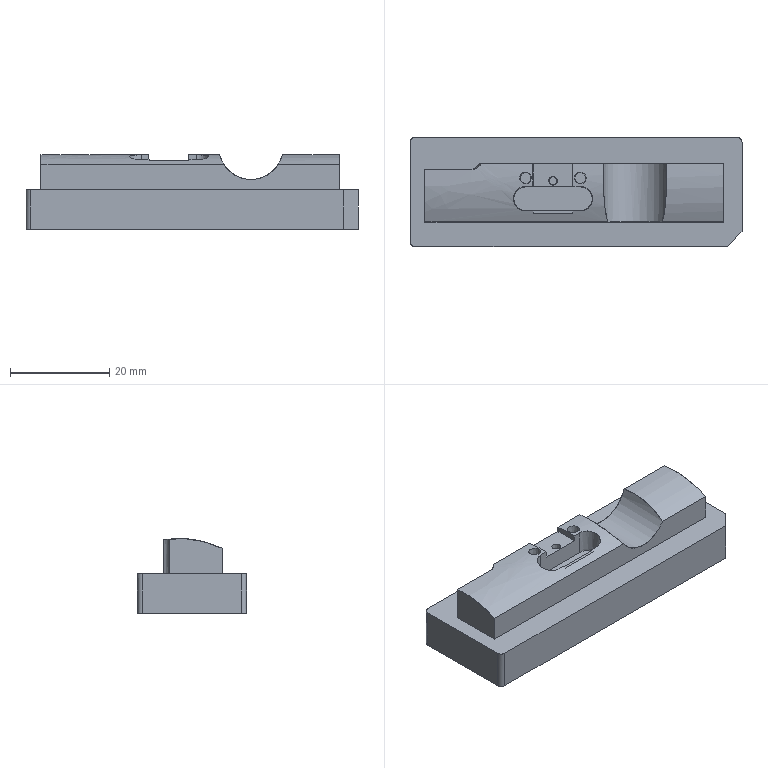NC program | PowerMill | posted with a generic post | part box 67 x 22 x 15.086 mm
Lines 39489 to 40021 of 148586:
N39586 M6
N39587 S8500 M03
N39588 G00 G90 X0.0 Y0.0
N39589 G43 Z9.7955 H3
N39590
N39591 G05 P10000 R8
N39592 X-35.7864 Y-21.1499
N39593 Z-6.09
N39594 G01 Z-7.29 F360.0
N39595 X-34.3023 Y-16.088 F600.0
N39596 X-24.7543 Y-11.314
N39597 X-30.4768
N39598 X-30.8691 Y-11.2993
N39599 X-31.2592 Y-11.2554
N39600 X-31.645 Y-11.1824
N39601 X-32.0242 Y-11.0808
N39602 X-32.3948 Y-10.9511
N39603 X-32.7546 Y-10.7941
N39604 X-33.1018 Y-10.6106
N39605 G02 X-33.7501 Y-10.1686 I3.1857 J5.3691
N39606 G01 X-34.0477 Y-9.9125
N39607 X-34.3253 Y-9.6349
N39608 G02 X-34.8145 Y-9.0214 I4.5048 J4.0941
N39609 G01 X-35.0234 Y-8.689
N39610 X-35.2068 Y-8.3419
N39611 X-35.3638 Y-7.9821
N39612 X-35.4935 Y-7.6115
N39613 X-35.5951 Y-7.2322
N39614 X-35.6681 Y-6.8465
N39615 X-35.7121 Y-6.4564
N39616 X-35.7267 Y-6.064
N39617 X-35.7268 Y4.5075
N39618 X-35.7121 Y4.8999
N39619 X-35.6681 Y5.29
N39620 X-35.5951 Y5.6758
N39621 X-35.4935 Y6.055
N39622 X-35.3638 Y6.4256
N39623 G02 X-35.0234 Y7.1326 I5.7015 J-2.3102
N39624 G01 X-34.8145 Y7.465
N39625 X-34.5814 Y7.7809
N39626 X-34.3253 Y8.0785
N39627 X-34.0477 Y8.3561
N39628 X-33.7501 Y8.6122
N39629 X-33.4342 Y8.8453
N39630 X-33.1017 Y9.0542
N39631 X-32.7547 Y9.2376
N39632 G02 X-32.0242 Y9.5243 I2.6199 J-5.6014
N39633 G01 X-31.645 Y9.6259
N39634 G02 X-30.8691 Y9.7429 I1.2931 J-5.9472
N39635 G01 X-30.4767 Y9.7575
N39636 X-23.1899
N39637 G03 X-22.5805 Y9.9646 I0.0 J1.0
N39638 G02 X-21.9467 Y10.3575 I3.3066 J-4.6275
N39639 G01 X-21.6205 Y10.5144
N39640 G02 X-20.5629 Y10.8499 I2.169 J-5.0017
N39641 G01 X-20.2312 Y10.9077
N39642 X-19.8712 Y10.9451
N39643 X-19.5093 Y10.9576
N39644 X29.7595 Y10.9575
N39645 X30.1518 Y10.9429
N39646 X30.542 Y10.8989
N39647 X30.9277 Y10.8259
N39648 X31.307 Y10.7243
N39649 X31.6775 Y10.5946
N39650 X32.0374 Y10.4376
N39651 G02 X32.7169 Y10.0453 I-2.6238 J-5.3293
N39652 G01 X33.0199 Y9.8224
N39653 X33.3304 Y9.5561
N39654 X33.608 Y9.2784
N39655 X33.8641 Y8.9809
N39656 X34.0973 Y8.665
N39657 X34.3061 Y8.3326
N39658 X34.4896 Y7.9854
N39659 X34.6466 Y7.6256
N39660 X34.7762 Y7.255
N39661 X34.8779 Y6.8758
N39662 X34.9509 Y6.49
N39663 X34.9948 Y6.0999
N39664 X35.0095 Y5.7076
N39665 Y-6.064
N39666 X34.9948 Y-6.4563
N39667 X34.9509 Y-6.8465
N39668 X34.8779 Y-7.2322
N39669 G02 X34.6466 Y-7.9821 I-6.0078 J1.4426
N39670 G01 X34.4896 Y-8.3419
N39671 X34.3061 Y-8.689
N39672 X34.0972 Y-9.0214
N39673 X33.8641 Y-9.3373
N39674 X33.608 Y-9.6349
N39675 X33.3304 Y-9.9125
N39676 X33.0328 Y-10.1686
N39677 X32.7169 Y-10.4018
N39678 X32.3845 Y-10.6106
N39679 X32.0374 Y-10.7941
N39680 G02 X31.307 Y-11.0808 I-2.6343 J5.6378
N39681 G01 X30.9277 Y-11.1824
N39682 G02 X30.1518 Y-11.2993 I-1.2836 J5.8835
N39683 G01 X29.7595 Y-11.314
N39684 X-24.7543
N39685 G00 Z9.7955
N39686 G05 P0
N39687 (---------------)
N39688 ( END TOOLPATH : 粗公基准台01-基准面偏置-D10 )
N39689 (---------------)
N39690 ( START TOOLPATH : 粗公基准台01-外形侧光-D10 )
N39691 (---------------)
N39692 G00 X0.0 Y0.0 Z10.795
N39693 G05 P10000 R8
N39694 X32.5724 Y-10.7005
N39695 Z-6.06
N39696 G01 Z-7.26 F360.0
N39697 G03 X31.4255 Y-10.65 I-0.6344 J-1.3593 F600.0
N39698 G02 X29.8166 Y-10.9437 I-1.6691 J4.5906
N39699 G01 X-0.3872 Y-10.9439
N39700 X-30.3333 Y-10.944
N39701 G02 X-35.3568 Y-5.9375 I-0.1343 J4.8887
N39702 G01 Y4.3892
N39703 G02 X-30.5914 Y9.3862 I4.8831 J0.114
N39704 G01 X-22.7836 Y9.3875
N39705 G03 X-22.6404 Y9.4405 I0.0 J0.2201
N39706 G02 X-19.4905 Y10.5876 I3.1435 J-3.7338
N39707 G01 X-0.5282 Y10.5874
N39708 X29.8197 Y10.5872
N39709 G02 X34.6395 Y5.6793 I-0.0604 J-4.88
N39710 G01 Y-5.9381
N39711 G02 X31.4255 Y-10.65 I-4.8831 J-0.1213
N39712 G03 X30.5788 Y-11.4254 I0.5125 J-1.4097
N39713 G01 X32.4404 Y-10.6877
N39714 G03 X31.2949 Y-10.6111 I-0.6652 J-1.3444
N39715 G02 X29.8166 Y-10.8637 I-1.5385 J4.5517
N39716 G01 X-0.3872 Y-10.864
N39717 X-30.3329
N39718 G02 X-35.2768 Y-5.9375 I-0.1347 J4.8087
N39719 G01 Y4.3886
N39720 G02 X-30.591 Y9.3062 I4.8031 J0.1146
N39721 G01 X-22.7836 Y9.3075
N39722 G03 X-22.5883 Y9.3798 I0.0 J0.3001
N39723 G02 X-19.4905 Y10.5076 I3.0912 J-3.6725
N39724 G01 X-0.5282 Y10.5074
N39725 X29.8166 Y10.5072
N39726 G02 X34.5595 Y5.6793 I-0.0573 J-4.7999
N39727 G01 Y-5.9375
N39728 G02 X31.2949 Y-10.6111 I-4.8031 J-0.1219
N39729 G03 X30.4307 Y-11.3669 I0.4803 J-1.421
N39730 G00 Z10.795
N39731 G05 P0
N39732 (---------------)
N39733 ( END TOOLPATH : 粗公基准台01-外形侧光-D10 )
N39734 (---------------)
N39735 ( START TOOLPATH : 粗公基准台01-基准台侧光-D10 )
N39736 (---------------)
N39737 G00 X0.0 Y0.0 Z9.7955
N39738 G05 P10000 R8
N39739 X37.757 Y-17.9972
N39740 Z-13.99
N39741 G01 Z-15.19 F360.0
N39742 G03 X34.2214 Y-14.4617 I-1.7678 J1.7678 F600.0
N39743 G01 X34.0275 Y-14.6556
N39744 X34.0263 Y-14.6567
N39745 X34.0251 Y-14.6579
N39746 X33.8608 Y-14.8093
N39747 X33.8591 Y-14.8109
N39748 X33.8573 Y-14.8124
N39749 X33.5746 Y-15.0439
N39750 X33.5723 Y-15.0457
N39751 X33.5699 Y-15.0474
N39752 X33.2627 Y-15.263
N39753 X33.261 Y-15.2642
N39754 X33.2591 Y-15.2654
N39755 X33.1193 Y-15.3527
N39756 X33.117 Y-15.3541
N39757 X33.1146 Y-15.3554
N39758 X32.6677 Y-15.5942
N39759 X32.6648 Y-15.5957
N39760 X32.6618 Y-15.597
N39761 X32.3835 Y-15.7179
N39762 X32.3818 Y-15.7186
N39763 X32.38 Y-15.7193
N39764 X32.2113 Y-15.7831
N39765 X32.2088 Y-15.784
N39766 X32.2063 Y-15.7848
N39767 X31.7594 Y-15.9214
N39768 X31.7558 Y-15.9224
N39769 X31.7522 Y-15.9232
N39770 X31.3052 Y-16.0157
N39771 X31.3016 Y-16.0164
N39772 X31.2981 Y-16.0169
N39773 X30.8511 Y-16.0678
N39774 X30.8476 Y-16.0681
N39775 X30.8441 Y-16.0683
N39776 X30.3971 Y-16.08
N39777 X30.3961
N39778 X30.395
N39779 X-32.183
N39780 X-32.1831
N39781 X-32.1833
N39782 X-32.6303 Y-16.0783
N39783 X-32.6326
N39784 X-32.6349 Y-16.0782
N39785 X-33.0819 Y-16.0506
N39786 X-33.0847 Y-16.0504
N39787 X-33.0874 Y-16.0501
N39788 X-33.5344 Y-15.9909
N39789 X-33.5376 Y-15.9904
N39790 X-33.5408 Y-15.9898
N39791 X-33.9878 Y-15.8935
N39792 X-33.9906 Y-15.8929
N39793 X-33.9933 Y-15.8921
N39794 X-34.4403 Y-15.7616
N39795 X-34.4434 Y-15.7606
N39796 X-34.4464 Y-15.7595
N39797 X-34.8934 Y-15.589
N39798 X-34.8965 Y-15.5877
N39799 X-34.8995 Y-15.5863
N39800 X-35.3465 Y-15.3718
N39801 X-35.3494 Y-15.3703
N39802 X-35.3523 Y-15.3687
N39803 X-35.7993 Y-15.1068
N39804 X-35.8023 Y-15.1049
N39805 X-35.8051 Y-15.103
N39806 X-36.21 Y-14.8158
N39807 X-36.213 Y-14.8136
N39808 X-36.2159 Y-14.8112
N39809 X-36.705 Y-14.3909
N39810 X-36.7083 Y-14.3879
N39811 X-36.7115 Y-14.3847
N39812 X-37.1507 Y-13.9109
N39813 X-37.1531 Y-13.9082
N39814 X-37.1554 Y-13.9054
N39815 X-37.5003 Y-13.4584
N39816 X-37.502 Y-13.4562
N39817 X-37.5035 Y-13.4539
N39818 X-37.6134 Y-13.289
N39819 X-37.6145 Y-13.2874
N39820 X-37.6155 Y-13.2857
N39821 X-37.7839 Y-13.0036
N39822 X-37.7851 Y-13.0015
N39823 X-37.7862 Y-12.9994
N39824 X-38.0179 Y-12.5524
N39825 X-38.0194 Y-12.5493
N39826 X-38.0208 Y-12.5461
N39827 X-38.2051 Y-12.0991
N39828 X-38.2062 Y-12.0962
N39829 X-38.2072 Y-12.0933
N39830 X-38.3524 Y-11.6463
N39831 X-38.3533 Y-11.6434
N39832 X-38.3541 Y-11.6403
N39833 X-38.4617 Y-11.1934
N39834 X-38.4623 Y-11.1907
N39835 X-38.4628 Y-11.1881
N39836 X-38.5196 Y-10.8544
N39837 X-38.5201 Y-10.8513
N39838 X-38.5204 Y-10.8483
N39839 X-38.5718 Y-10.288
N39840 X-38.572 Y-10.285
N39841 X-38.5721 Y-10.2821
N39842 X-38.58 Y-9.8351
N39843 Y-9.8344
N39844 Y-9.8337
N39845 Y9.8337
N39846 Y9.8344
N39847 Y9.8351
N39848 X-38.5721 Y10.2821
N39849 X-38.572 Y10.2847
N39850 X-38.5719 Y10.2872
N39851 X-38.5351 Y10.7342
N39852 X-38.5348 Y10.7373
N39853 X-38.5344 Y10.7403
N39854 X-38.4629 Y11.1873
N39855 X-38.4624 Y11.1903
N39856 X-38.4617 Y11.1934
N39857 X-38.3541 Y11.6403
N39858 X-38.3533 Y11.6434
N39859 X-38.3524 Y11.6463
N39860 X-38.2072 Y12.0933
N39861 X-38.2062 Y12.0962
N39862 X-38.2051 Y12.0991
N39863 X-38.0208 Y12.5461
N39864 X-38.0194 Y12.5493
N39865 X-38.0179 Y12.5524
N39866 X-37.7862 Y12.9994
N39867 X-37.7851 Y13.0015
N39868 X-37.7839 Y13.0036
N39869 X-37.6155 Y13.2857
N39870 X-37.6145 Y13.2874
N39871 X-37.6134 Y13.289
N39872 X-37.5035 Y13.4539
N39873 X-37.502 Y13.4562
N39874 X-37.5003 Y13.4584
N39875 X-37.1632 Y13.8962
N39876 X-37.161 Y13.8989
N39877 X-37.1587 Y13.9015
N39878 X-36.7396 Y14.3577
N39879 X-36.7365 Y14.3609
N39880 X-36.7332 Y14.3639
N39881 X-36.2584 Y14.7775
N39882 X-36.2555 Y14.7799
N39883 X-36.2525 Y14.7822
N39884 X-35.8055 Y15.1027
N39885 X-35.8024 Y15.1048
N39886 X-35.7993 Y15.1068
N39887 X-35.3523 Y15.3687
N39888 X-35.3494 Y15.3703
N39889 X-35.3465 Y15.3718
N39890 X-34.8995 Y15.5863
N39891 X-34.8965 Y15.5877
N39892 X-34.8934 Y15.589
N39893 X-34.4464 Y15.7595
N39894 X-34.4434 Y15.7606
N39895 X-34.4403 Y15.7616
N39896 X-33.9933 Y15.8921
N39897 X-33.9906 Y15.8929
N39898 X-33.9878 Y15.8935
N39899 X-33.5408 Y15.9898
N39900 X-33.5376 Y15.9904
N39901 X-33.5344 Y15.9909
N39902 X-33.0874 Y16.0501
N39903 X-33.0847 Y16.0504
N39904 X-33.0819 Y16.0506
N39905 X-32.6349 Y16.0782
N39906 X-32.6326 Y16.0783
N39907 X-32.6303
N39908 X-32.1833 Y16.08
N39909 X-32.1831
N39910 X-32.183
N39911 X0.0
N39912 X32.183
N39913 X32.1831
N39914 X32.1833
N39915 X32.6303 Y16.0783
N39916 X32.6326
N39917 X32.6349 Y16.0782
N39918 X33.0819 Y16.0506
N39919 X33.0847 Y16.0504
N39920 X33.0874 Y16.0501
N39921 X33.5344 Y15.9909
N39922 X33.5376 Y15.9904
N39923 X33.5408 Y15.9898
N39924 X33.9878 Y15.8935
N39925 X33.9906 Y15.8929
N39926 X33.9933 Y15.8921
N39927 X34.4403 Y15.7616
N39928 X34.4434 Y15.7606
N39929 X34.4464 Y15.7595
N39930 X34.8934 Y15.589
N39931 X34.8965 Y15.5877
N39932 X34.8995 Y15.5863
N39933 X35.3465 Y15.3718
N39934 X35.3494 Y15.3703
N39935 X35.3523 Y15.3687
N39936 X35.7993 Y15.1068
N39937 X35.8023 Y15.1049
N39938 X35.8051 Y15.103
N39939 X36.21 Y14.8158
N39940 X36.213 Y14.8136
N39941 X36.2159 Y14.8112
N39942 X36.705 Y14.3909
N39943 X36.7083 Y14.3879
N39944 X36.7115 Y14.3847
N39945 X37.1507 Y13.9109
N39946 X37.1531 Y13.9082
N39947 X37.1554 Y13.9054
N39948 X37.5003 Y13.4584
N39949 X37.502 Y13.4562
N39950 X37.5035 Y13.4539
N39951 X37.6134 Y13.289
N39952 X37.6145 Y13.2874
N39953 X37.6155 Y13.2857
N39954 X37.7839 Y13.0036
N39955 X37.7851 Y13.0015
N39956 X37.7862 Y12.9994
N39957 X38.0179 Y12.5524
N39958 X38.0194 Y12.5493
N39959 X38.0208 Y12.5461
N39960 X38.2051 Y12.0991
N39961 X38.2062 Y12.0962
N39962 X38.2072 Y12.0933
N39963 X38.3524 Y11.6463
N39964 X38.3533 Y11.6434
N39965 X38.3541 Y11.6403
N39966 X38.4617 Y11.1934
N39967 X38.4623 Y11.1907
N39968 X38.4628 Y11.1881
N39969 X38.5196 Y10.8544
N39970 X38.5201 Y10.8513
N39971 X38.5204 Y10.8483
N39972 X38.5718 Y10.288
N39973 X38.572 Y10.285
N39974 X38.5721 Y10.2821
N39975 X38.58 Y9.8351
N39976 Y9.8344
N39977 Y9.8337
N39978 X38.5798 Y-8.0457
N39979 Y-8.0479
N39980 X38.5797 Y-8.05
N39981 X38.5556 Y-8.497
N39982 X38.5553 Y-8.5006
N39983 X38.5549 Y-8.5042
N39984 X38.4901 Y-8.9512
N39985 X38.4895 Y-8.9548
N39986 X38.4887 Y-8.9583
N39987 X38.3817 Y-9.4053
N39988 X38.3807 Y-9.4089
N39989 X38.3796 Y-9.4125
N39990 X38.2274 Y-9.8595
N39991 X38.226 Y-9.8631
N39992 X38.2245 Y-9.8666
N39993 X38.0225 Y-10.3136
N39994 X38.0207 Y-10.3173
N39995 X38.0188 Y-10.3208
N39996 X37.7597 Y-10.7678
N39997 X37.7581 Y-10.7704
N39998 X37.7564 Y-10.773
N39999 X37.6127 Y-10.9819
N40000 X37.6114 Y-10.9837
N40001 X37.6101 Y-10.9855
N40002 X37.4262 Y-11.2235
N40003 X37.4245 Y-11.2257
N40004 X37.4226 Y-11.2278
N40005 X37.1596 Y-11.5233
N40006 X37.158 Y-11.525
N40007 X37.1564 Y-11.5267
N40008 X34.2214 Y-14.4617
N40009 G03 X37.757 Y-17.9972 I1.7678 J-1.7677
N40010 G01 X37.7112 Y-17.9298
N40011 G03 X34.1756 Y-14.3943 I-1.7678 J1.7677
N40012 G01 X33.9709 Y-14.599
N40013 X33.8066 Y-14.7505
N40014 X33.5239 Y-14.982
N40015 X33.2168 Y-15.1975
N40016 X33.0769 Y-15.2848
N40017 X32.63 Y-15.5237
N40018 X32.3517 Y-15.6445
N40019 X32.183 Y-15.7083
N40020 X31.736 Y-15.8449
N40021 X31.289 Y-15.9374
N40022 X30.842 Y-15.9883
N40023 X30.395 Y-16.0
N40024 X-32.183
N40025 X-32.63 Y-15.9983
N40026 X-33.0769 Y-15.9708
N40027 X-33.5239 Y-15.9116
N40028 X-33.9709 Y-15.8153
N40029 X-34.4179 Y-15.6848
N40030 X-34.8649 Y-15.5142
N40031 X-35.3119 Y-15.2997
N40032 X-35.7589 Y-15.0377
N40033 X-36.1637 Y-14.7505
N40034 X-36.6528 Y-14.3303
N40035 X-37.0921 Y-13.8566
N40036 X-37.437 Y-13.4096
N40037 X-37.5468 Y-13.2447
N40038 X-37.7152 Y-12.9626
N40039 X-37.9468 Y-12.5156
N40040 X-38.1311 Y-12.0686
N40041 X-38.2763 Y-11.6216
N40042 X-38.3839 Y-11.1746
N40043 X-38.4408 Y-10.841
N40044 X-38.4921 Y-10.2807
N40045 X-38.5 Y-9.8337
N40046 Y9.8337
N40047 X-38.4921 Y10.2807
N40048 X-38.4554 Y10.7277
N40049 X-38.3839 Y11.1746
N40050 X-38.2763 Y11.6216
N40051 X-38.1311 Y12.0686
N40052 X-37.9468 Y12.5156
N40053 X-37.7152 Y12.9626
N40054 X-37.5468 Y13.2447
N40055 X-37.437 Y13.4096
N40056 X-37.0998 Y13.8474
N40057 X-36.6807 Y14.3035
N40058 X-36.2058 Y14.7172
N40059 X-35.7589 Y15.0377
N40060 X-35.3119 Y15.2997
N40061 X-34.8649 Y15.5142
N40062 X-34.4179 Y15.6848
N40063 X-33.9709 Y15.8153
N40064 X-33.5239 Y15.9116
N40065 X-33.0769 Y15.9708
N40066 X-32.63 Y15.9983
N40067 X-32.183 Y16.0
N40068 X0.0
N40069 X32.183
N40070 X32.63 Y15.9983
N40071 X33.0769 Y15.9708
N40072 X33.5239 Y15.9116
N40073 X33.9709 Y15.8153
N40074 X34.4179 Y15.6848
N40075 X34.8649 Y15.5142
N40076 X35.3119 Y15.2997
N40077 X35.7589 Y15.0377
N40078 X36.1637 Y14.7505
N40079 X36.6528 Y14.3303
N40080 X37.0921 Y13.8566
N40081 X37.437 Y13.4096
N40082 X37.5468 Y13.2447
N40083 X37.7152 Y12.9626
N40084 X37.9468 Y12.5156
N40085 X38.1311 Y12.0686
N40086 X38.2763 Y11.6216
N40087 X38.3839 Y11.1746
N40088 X38.4408 Y10.841
N40089 X38.4921 Y10.2807
N40090 X38.5 Y9.8337
N40091 X38.4998 Y-8.0457
N40092 X38.4757 Y-8.4927
N40093 X38.4109 Y-8.9397
N40094 X38.3039 Y-9.3867
N40095 X38.1516 Y-9.8337
N40096 X37.9496 Y-10.2807
N40097 X37.6905 Y-10.7277
N40098 X37.5468 Y-10.9366
N40099 X37.3629 Y-11.1746
N40100 X37.0998 Y-11.4701
N40101 X34.1756 Y-14.3943
N40102 G03 X37.7112 Y-17.9298 I1.7678 J-1.7678
N40103 G00 Z9.7955
N40104 G05 P0
N40105 (---------------)
N40106 ( END TOOLPATH : 粗公基准台01-基准台侧光-D10 )
N40107 (---------------)
N40108
N40109 M05
N40110 G53 Z0.0
N40111 (---------------)
N40112 ( START TOOLPATH : 粗公精光01-平行-R1.5 )
N40113 (---------------)
N40114 ( TOOL NO.    :22 )
N40115 ( TOOL TYPE   : BALLNOSED)
N40116 ( TOOL ID     : R1.5_1_1)
N40117 ( TOOL DIA    : 3.0 LENGTH 60.28)
N40118 T22